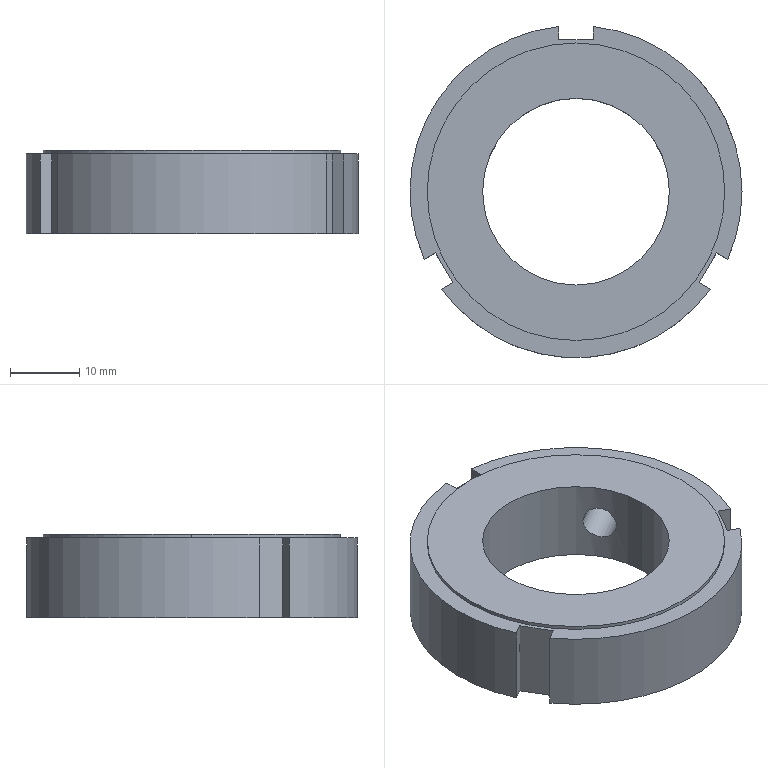Part | STEP file | PN_0019_default | 1 solid | 22 faces | box 48 x 47.869 x 12 mm | volume 14121 mm3 | plane 12 | cylinder 10 | commonest cylinder face diameters 48 x4 5 x2 27 x2 43 x2